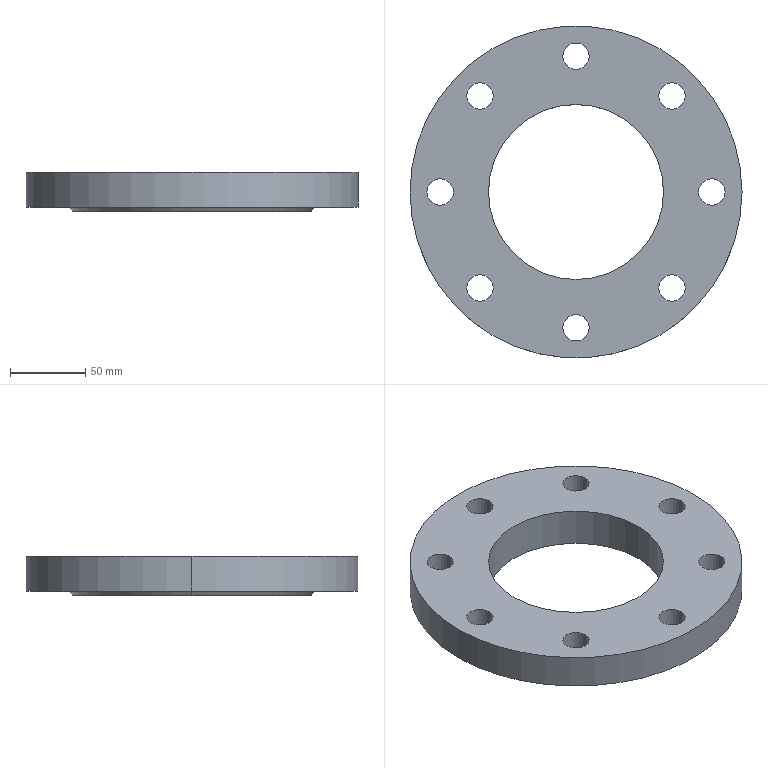Part | SolidWorks | features Extrusion 1, ICE 1, RefAxis 1, RevCut 1 | 1 solid | 25 faces | box 220 x 220 x 26 mm | volume 615594 mm3 | cylinder 20 | plane 3 | cone 2 | commonest cylinder face diameters 17.5 x16 116 x2 220 x2
STEP:
#1=CARTESIAN_POINT('',(-79.,0.,0.));
#2=VERTEX_POINT('',#1);
#3=CARTESIAN_POINT('',(79.,0.,0.));
#4=VERTEX_POINT('',#3);
#5=CARTESIAN_POINT('',(0.,0.,0.));
#6=DIRECTION('',(0.,0.,-1.));
#7=DIRECTION('',(-1.,0.,0.));
#8=AXIS2_PLACEMENT_3D('',#5,#6,#7);
#9=CIRCLE('',#8,79.);
#10=EDGE_CURVE('',#2,#4,#9,.T.);
#11=ORIENTED_EDGE('',*,*,#10,.F.);
#12=CARTESIAN_POINT('',(-81.,0.,3.));
#13=VERTEX_POINT('',#12);
#14=CARTESIAN_POINT('',(-79.,0.,0.));
#15=DIRECTION('',(-0.5547,0.,0.8321));
#16=VECTOR('',#15,1000.);
#17=LINE('',#14,#16);
#18=EDGE_CURVE('',#2,#13,#17,.T.);
#19=ORIENTED_EDGE('',*,*,#18,.T.);
#20=CARTESIAN_POINT('',(81.,0.,3.));
#21=VERTEX_POINT('',#20);
#22=CARTESIAN_POINT('',(0.,0.,3.));
#23=DIRECTION('',(0.,0.,-1.));
#24=DIRECTION('',(-1.,0.,0.));
#25=AXIS2_PLACEMENT_3D('',#22,#23,#24);
#26=CIRCLE('',#25,81.);
#27=EDGE_CURVE('',#13,#21,#26,.T.);
#28=ORIENTED_EDGE('',*,*,#27,.T.);
#29=CARTESIAN_POINT('',(79.,0.,0.));
#30=DIRECTION('',(0.5547,0.,0.8321));
#31=VECTOR('',#30,1000.);
#32=LINE('',#29,#31);
#33=EDGE_CURVE('',#4,#21,#32,.T.);
#34=ORIENTED_EDGE('',*,*,#33,.F.);
#35=EDGE_LOOP('',(#11,#19,#28,#34));
#36=FACE_OUTER_BOUND('',#35,.T.);
#37=CARTESIAN_POINT('',(0.,0.,0.));
#38=DIRECTION('',(0.,0.,1.));
#39=DIRECTION('',(1.,0.,0.));
#40=AXIS2_PLACEMENT_3D('',#37,#38,#39);
#41=CONICAL_SURFACE('',#40,79.,0.588);
#42=ADVANCED_FACE('',(#36),#41,.T.);
#43=CARTESIAN_POINT('',(-58.,0.,0.));
#44=VERTEX_POINT('',#43);
#45=CARTESIAN_POINT('',(58.,0.,0.));
#46=VERTEX_POINT('',#45);
#47=CARTESIAN_POINT('',(0.,0.,0.));
#48=DIRECTION('',(0.,0.,1.));
#49=DIRECTION('',(1.,0.,0.));
#50=AXIS2_PLACEMENT_3D('',#47,#48,#49);
#51=CIRCLE('',#50,58.);
#52=EDGE_CURVE('',#44,#46,#51,.T.);
#53=ORIENTED_EDGE('',*,*,#52,.F.);
#54=CARTESIAN_POINT('',(-58.,0.,26.));
#55=VERTEX_POINT('',#54);
#56=CARTESIAN_POINT('',(-58.,0.,0.));
#57=DIRECTION('',(0.,0.,1.));
#58=VECTOR('',#57,1000.);
#59=LINE('',#56,#58);
#60=EDGE_CURVE('',#44,#55,#59,.T.);
#61=ORIENTED_EDGE('',*,*,#60,.T.);
#62=CARTESIAN_POINT('',(58.,0.,26.));
#63=VERTEX_POINT('',#62);
#64=CARTESIAN_POINT('',(0.,0.,26.));
#65=DIRECTION('',(0.,0.,1.));
#66=DIRECTION('',(1.,0.,0.));
#67=AXIS2_PLACEMENT_3D('',#64,#65,#66);
#68=CIRCLE('',#67,58.);
#69=EDGE_CURVE('',#55,#63,#68,.T.);
#70=ORIENTED_EDGE('',*,*,#69,.T.);
#71=CARTESIAN_POINT('',(58.,0.,0.));
#72=DIRECTION('',(0.,0.,1.));
#73=VECTOR('',#72,1000.);
#74=LINE('',#71,#73);
#75=EDGE_CURVE('',#46,#63,#74,.T.);
#76=ORIENTED_EDGE('',*,*,#75,.F.);
#77=EDGE_LOOP('',(#53,#61,#70,#76));
#78=FACE_OUTER_BOUND('',#77,.T.);
#79=CARTESIAN_POINT('',(0.,0.,0.));
#80=DIRECTION('',(0.,0.,1.));
#81=DIRECTION('',(1.,0.,0.));
#82=AXIS2_PLACEMENT_3D('',#79,#80,#81);
#83=CYLINDRICAL_SURFACE('',#82,58.);
#84=ADVANCED_FACE('',(#78),#83,.F.);
#85=CARTESIAN_POINT('',(-72.39,63.64,26.));
#86=VERTEX_POINT('',#85);
#87=CARTESIAN_POINT('',(-54.89,63.64,26.));
#88=VERTEX_POINT('',#87);
#89=CARTESIAN_POINT('',(-63.64,63.64,26.));
#90=DIRECTION('',(0.,0.,1.));
#91=DIRECTION('',(1.,0.,0.));
#92=AXIS2_PLACEMENT_3D('',#89,#90,#91);
#93=CIRCLE('',#92,8.75);
#94=EDGE_CURVE('',#86,#88,#93,.T.);
#95=ORIENTED_EDGE('',*,*,#94,.T.);
#96=CARTESIAN_POINT('',(-54.89,63.64,3.));
#97=VERTEX_POINT('',#96);
#98=CARTESIAN_POINT('',(-54.89,63.64,26.));
#99=DIRECTION('',(0.,0.,-1.));
#100=VECTOR('',#99,1000.);
#101=LINE('',#98,#100);
#102=EDGE_CURVE('',#88,#97,#101,.T.);
#103=ORIENTED_EDGE('',*,*,#102,.T.);
#104=CARTESIAN_POINT('',(-72.39,63.64,3.));
#105=VERTEX_POINT('',#104);
#106=CARTESIAN_POINT('',(-63.64,63.64,3.));
#107=DIRECTION('',(0.,0.,-1.));
#108=DIRECTION('',(-1.,0.,0.));
#109=AXIS2_PLACEMENT_3D('',#106,#107,#108);
#110=CIRCLE('',#109,8.75);
#111=EDGE_CURVE('',#97,#105,#110,.T.);
#112=ORIENTED_EDGE('',*,*,#111,.T.);
#113=CARTESIAN_POINT('',(-72.39,63.64,26.));
#114=DIRECTION('',(0.,0.,-1.));
#115=VECTOR('',#114,1000.);
#116=LINE('',#113,#115);
#117=EDGE_CURVE('',#86,#105,#116,.T.);
#118=ORIENTED_EDGE('',*,*,#117,.F.);
#119=EDGE_LOOP('',(#95,#103,#112,#118));
#120=FACE_OUTER_BOUND('',#119,.T.);
#121=CARTESIAN_POINT('',(-63.64,63.64,26.));
#122=DIRECTION('',(0.,0.,-1.));
#123=DIRECTION('',(-1.,0.,0.));
#124=AXIS2_PLACEMENT_3D('',#121,#122,#123);
#125=CYLINDRICAL_SURFACE('',#124,8.75);
#126=ADVANCED_FACE('',(#120),#125,.F.);
#127=CARTESIAN_POINT('',(-98.75,0.,26.));
#128=VERTEX_POINT('',#127);
#129=CARTESIAN_POINT('',(-81.25,0.,26.));
#130=VERTEX_POINT('',#129);
#131=CARTESIAN_POINT('',(-90.,0.,26.));
#132=DIRECTION('',(0.,0.,1.));
#133=DIRECTION('',(1.,0.,0.));
#134=AXIS2_PLACEMENT_3D('',#131,#132,#133);
#135=CIRCLE('',#134,8.75);
#136=EDGE_CURVE('',#128,#130,#135,.T.);
#137=ORIENTED_EDGE('',*,*,#136,.T.);
#138=CARTESIAN_POINT('',(-81.25,0.,3.));
#139=VERTEX_POINT('',#138);
#140=CARTESIAN_POINT('',(-81.25,0.,26.));
#141=DIRECTION('',(0.,0.,-1.));
#142=VECTOR('',#141,1000.);
#143=LINE('',#140,#142);
#144=EDGE_CURVE('',#130,#139,#143,.T.);
#145=ORIENTED_EDGE('',*,*,#144,.T.);
#146=CARTESIAN_POINT('',(-98.75,0.,3.));
#147=VERTEX_POINT('',#146);
#148=CARTESIAN_POINT('',(-90.,0.,3.));
#149=DIRECTION('',(0.,0.,-1.));
#150=DIRECTION('',(-1.,0.,0.));
#151=AXIS2_PLACEMENT_3D('',#148,#149,#150);
#152=CIRCLE('',#151,8.75);
#153=EDGE_CURVE('',#139,#147,#152,.T.);
#154=ORIENTED_EDGE('',*,*,#153,.T.);
#155=CARTESIAN_POINT('',(-98.75,0.,26.));
#156=DIRECTION('',(0.,0.,-1.));
#157=VECTOR('',#156,1000.);
#158=LINE('',#155,#157);
#159=EDGE_CURVE('',#128,#147,#158,.T.);
#160=ORIENTED_EDGE('',*,*,#159,.F.);
#161=EDGE_LOOP('',(#137,#145,#154,#160));
#162=FACE_OUTER_BOUND('',#161,.T.);
#163=CARTESIAN_POINT('',(-90.,0.,26.));
#164=DIRECTION('',(0.,0.,-1.));
#165=DIRECTION('',(-1.,0.,0.));
#166=AXIS2_PLACEMENT_3D('',#163,#164,#165);
#167=CYLINDRICAL_SURFACE('',#166,8.75);
#168=ADVANCED_FACE('',(#162),#167,.F.);
#169=CARTESIAN_POINT('',(-72.39,-63.64,26.));
#170=VERTEX_POINT('',#169);
#171=CARTESIAN_POINT('',(-54.89,-63.64,26.));
#172=VERTEX_POINT('',#171);
#173=CARTESIAN_POINT('',(-63.64,-63.64,26.));
#174=DIRECTION('',(0.,0.,1.));
#175=DIRECTION('',(1.,0.,0.));
#176=AXIS2_PLACEMENT_3D('',#173,#174,#175);
#177=CIRCLE('',#176,8.75);
#178=EDGE_CURVE('',#170,#172,#177,.T.);
#179=ORIENTED_EDGE('',*,*,#178,.T.);
#180=CARTESIAN_POINT('',(-54.89,-63.64,3.));
#181=VERTEX_POINT('',#180);
#182=CARTESIAN_POINT('',(-54.89,-63.64,26.));
#183=DIRECTION('',(0.,0.,-1.));
#184=VECTOR('',#183,1000.);
#185=LINE('',#182,#184);
#186=EDGE_CURVE('',#172,#181,#185,.T.);
#187=ORIENTED_EDGE('',*,*,#186,.T.);
#188=CARTESIAN_POINT('',(-72.39,-63.64,3.));
#189=VERTEX_POINT('',#188);
#190=CARTESIAN_POINT('',(-63.64,-63.64,3.));
#191=DIRECTION('',(0.,0.,-1.));
#192=DIRECTION('',(-1.,0.,0.));
#193=AXIS2_PLACEMENT_3D('',#190,#191,#192);
#194=CIRCLE('',#193,8.75);
#195=EDGE_CURVE('',#181,#189,#194,.T.);
#196=ORIENTED_EDGE('',*,*,#195,.T.);
#197=CARTESIAN_POINT('',(-72.39,-63.64,26.));
#198=DIRECTION('',(0.,0.,-1.));
#199=VECTOR('',#198,1000.);
#200=LINE('',#197,#199);
#201=EDGE_CURVE('',#170,#189,#200,.T.);
#202=ORIENTED_EDGE('',*,*,#201,.F.);
#203=EDGE_LOOP('',(#179,#187,#196,#202));
#204=FACE_OUTER_BOUND('',#203,.T.);
#205=CARTESIAN_POINT('',(-63.64,-63.64,26.));
#206=DIRECTION('',(0.,0.,-1.));
#207=DIRECTION('',(-1.,0.,0.));
#208=AXIS2_PLACEMENT_3D('',#205,#206,#207);
#209=CYLINDRICAL_SURFACE('',#208,8.75);
#210=ADVANCED_FACE('',(#204),#209,.F.);
#211=CARTESIAN_POINT('',(-8.75,-90.,26.));
#212=VERTEX_POINT('',#211);
#213=CARTESIAN_POINT('',(8.75,-90.,26.));
#214=VERTEX_POINT('',#213);
#215=CARTESIAN_POINT('',(0.,-90.,26.));
#216=DIRECTION('',(0.,0.,1.));
#217=DIRECTION('',(1.,0.,0.));
#218=AXIS2_PLACEMENT_3D('',#215,#216,#217);
#219=CIRCLE('',#218,8.75);
#220=EDGE_CURVE('',#212,#214,#219,.T.);
#221=ORIENTED_EDGE('',*,*,#220,.T.);
#222=CARTESIAN_POINT('',(8.75,-90.,3.));
#223=VERTEX_POINT('',#222);
#224=CARTESIAN_POINT('',(8.75,-90.,26.));
#225=DIRECTION('',(0.,0.,-1.));
#226=VECTOR('',#225,1000.);
#227=LINE('',#224,#226);
#228=EDGE_CURVE('',#214,#223,#227,.T.);
#229=ORIENTED_EDGE('',*,*,#228,.T.);
#230=CARTESIAN_POINT('',(-8.75,-90.,3.));
#231=VERTEX_POINT('',#230);
#232=CARTESIAN_POINT('',(0.,-90.,3.));
#233=DIRECTION('',(0.,0.,-1.));
#234=DIRECTION('',(-1.,0.,0.));
#235=AXIS2_PLACEMENT_3D('',#232,#233,#234);
#236=CIRCLE('',#235,8.75);
#237=EDGE_CURVE('',#223,#231,#236,.T.);
#238=ORIENTED_EDGE('',*,*,#237,.T.);
#239=CARTESIAN_POINT('',(-8.75,-90.,26.));
#240=DIRECTION('',(0.,0.,-1.));
#241=VECTOR('',#240,1000.);
#242=LINE('',#239,#241);
#243=EDGE_CURVE('',#212,#231,#242,.T.);
#244=ORIENTED_EDGE('',*,*,#243,.F.);
#245=EDGE_LOOP('',(#221,#229,#238,#244));
#246=FACE_OUTER_BOUND('',#245,.T.);
#247=CARTESIAN_POINT('',(0.,-90.,26.));
#248=DIRECTION('',(0.,0.,-1.));
#249=DIRECTION('',(-1.,0.,0.));
#250=AXIS2_PLACEMENT_3D('',#247,#248,#249);
#251=CYLINDRICAL_SURFACE('',#250,8.75);
#252=ADVANCED_FACE('',(#246),#251,.F.);
#253=CARTESIAN_POINT('',(54.89,-63.64,26.));
#254=VERTEX_POINT('',#253);
#255=CARTESIAN_POINT('',(72.39,-63.64,26.));
#256=VERTEX_POINT('',#255);
#257=CARTESIAN_POINT('',(63.64,-63.64,26.));
#258=DIRECTION('',(0.,0.,1.));
#259=DIRECTION('',(1.,0.,0.));
#260=AXIS2_PLACEMENT_3D('',#257,#258,#259);
#261=CIRCLE('',#260,8.75);
#262=EDGE_CURVE('',#254,#256,#261,.T.);
#263=ORIENTED_EDGE('',*,*,#262,.T.);
#264=CARTESIAN_POINT('',(72.39,-63.64,3.));
#265=VERTEX_POINT('',#264);
#266=CARTESIAN_POINT('',(72.39,-63.64,26.));
#267=DIRECTION('',(0.,0.,-1.));
#268=VECTOR('',#267,1000.);
#269=LINE('',#266,#268);
#270=EDGE_CURVE('',#256,#265,#269,.T.);
#271=ORIENTED_EDGE('',*,*,#270,.T.);
#272=CARTESIAN_POINT('',(54.89,-63.64,3.));
#273=VERTEX_POINT('',#272);
#274=CARTESIAN_POINT('',(63.64,-63.64,3.));
#275=DIRECTION('',(0.,0.,-1.));
#276=DIRECTION('',(-1.,0.,0.));
#277=AXIS2_PLACEMENT_3D('',#274,#275,#276);
#278=CIRCLE('',#277,8.75);
#279=EDGE_CURVE('',#265,#273,#278,.T.);
#280=ORIENTED_EDGE('',*,*,#279,.T.);
#281=CARTESIAN_POINT('',(54.89,-63.64,26.));
#282=DIRECTION('',(0.,0.,-1.));
#283=VECTOR('',#282,1000.);
#284=LINE('',#281,#283);
#285=EDGE_CURVE('',#254,#273,#284,.T.);
#286=ORIENTED_EDGE('',*,*,#285,.F.);
#287=EDGE_LOOP('',(#263,#271,#280,#286));
#288=FACE_OUTER_BOUND('',#287,.T.);
#289=CARTESIAN_POINT('',(63.64,-63.64,26.));
#290=DIRECTION('',(0.,0.,-1.));
#291=DIRECTION('',(-1.,0.,0.));
#292=AXIS2_PLACEMENT_3D('',#289,#290,#291);
#293=CYLINDRICAL_SURFACE('',#292,8.75);
#294=ADVANCED_FACE('',(#288),#293,.F.);
#295=CARTESIAN_POINT('',(81.25,0.,26.));
#296=VERTEX_POINT('',#295);
#297=CARTESIAN_POINT('',(98.75,0.,26.));
#298=VERTEX_POINT('',#297);
#299=CARTESIAN_POINT('',(90.,0.,26.));
#300=DIRECTION('',(0.,0.,1.));
#301=DIRECTION('',(1.,0.,0.));
#302=AXIS2_PLACEMENT_3D('',#299,#300,#301);
#303=CIRCLE('',#302,8.75);
#304=EDGE_CURVE('',#296,#298,#303,.T.);
#305=ORIENTED_EDGE('',*,*,#304,.T.);
#306=CARTESIAN_POINT('',(98.75,0.,3.));
#307=VERTEX_POINT('',#306);
#308=CARTESIAN_POINT('',(98.75,0.,26.));
#309=DIRECTION('',(0.,0.,-1.));
#310=VECTOR('',#309,1000.);
#311=LINE('',#308,#310);
#312=EDGE_CURVE('',#298,#307,#311,.T.);
#313=ORIENTED_EDGE('',*,*,#312,.T.);
#314=CARTESIAN_POINT('',(81.25,0.,3.));
#315=VERTEX_POINT('',#314);
#316=CARTESIAN_POINT('',(90.,0.,3.));
#317=DIRECTION('',(0.,0.,-1.));
#318=DIRECTION('',(-1.,0.,0.));
#319=AXIS2_PLACEMENT_3D('',#316,#317,#318);
#320=CIRCLE('',#319,8.75);
#321=EDGE_CURVE('',#307,#315,#320,.T.);
#322=ORIENTED_EDGE('',*,*,#321,.T.);
#323=CARTESIAN_POINT('',(81.25,0.,26.));
#324=DIRECTION('',(0.,0.,-1.));
#325=VECTOR('',#324,1000.);
#326=LINE('',#323,#325);
#327=EDGE_CURVE('',#296,#315,#326,.T.);
#328=ORIENTED_EDGE('',*,*,#327,.F.);
#329=EDGE_LOOP('',(#305,#313,#322,#328));
#330=FACE_OUTER_BOUND('',#329,.T.);
#331=CARTESIAN_POINT('',(90.,0.,26.));
#332=DIRECTION('',(0.,0.,-1.));
#333=DIRECTION('',(-1.,0.,0.));
#334=AXIS2_PLACEMENT_3D('',#331,#332,#333);
#335=CYLINDRICAL_SURFACE('',#334,8.75);
#336=ADVANCED_FACE('',(#330),#335,.F.);
#337=CARTESIAN_POINT('',(54.89,63.64,26.));
#338=VERTEX_POINT('',#337);
#339=CARTESIAN_POINT('',(72.39,63.64,26.));
#340=VERTEX_POINT('',#339);
#341=CARTESIAN_POINT('',(63.64,63.64,26.));
#342=DIRECTION('',(0.,0.,1.));
#343=DIRECTION('',(1.,0.,0.));
#344=AXIS2_PLACEMENT_3D('',#341,#342,#343);
#345=CIRCLE('',#344,8.75);
#346=EDGE_CURVE('',#338,#340,#345,.T.);
#347=ORIENTED_EDGE('',*,*,#346,.T.);
#348=CARTESIAN_POINT('',(72.39,63.64,3.));
#349=VERTEX_POINT('',#348);
#350=CARTESIAN_POINT('',(72.39,63.64,26.));
#351=DIRECTION('',(0.,0.,-1.));
#352=VECTOR('',#351,1000.);
#353=LINE('',#350,#352);
#354=EDGE_CURVE('',#340,#349,#353,.T.);
#355=ORIENTED_EDGE('',*,*,#354,.T.);
#356=CARTESIAN_POINT('',(54.89,63.64,3.));
#357=VERTEX_POINT('',#356);
#358=CARTESIAN_POINT('',(63.64,63.64,3.));
#359=DIRECTION('',(0.,0.,-1.));
#360=DIRECTION('',(-1.,0.,0.));
#361=AXIS2_PLACEMENT_3D('',#358,#359,#360);
#362=CIRCLE('',#361,8.75);
#363=EDGE_CURVE('',#349,#357,#362,.T.);
#364=ORIENTED_EDGE('',*,*,#363,.T.);
#365=CARTESIAN_POINT('',(54.89,63.64,26.));
#366=DIRECTION('',(0.,0.,-1.));
#367=VECTOR('',#366,1000.);
#368=LINE('',#365,#367);
#369=EDGE_CURVE('',#338,#357,#368,.T.);
#370=ORIENTED_EDGE('',*,*,#369,.F.);
#371=EDGE_LOOP('',(#347,#355,#364,#370));
#372=FACE_OUTER_BOUND('',#371,.T.);
#373=CARTESIAN_POINT('',(63.64,63.64,26.));
#374=DIRECTION('',(0.,0.,-1.));
#375=DIRECTION('',(-1.,0.,0.));
#376=AXIS2_PLACEMENT_3D('',#373,#374,#375);
#377=CYLINDRICAL_SURFACE('',#376,8.75);
#378=ADVANCED_FACE('',(#372),#377,.F.);
#379=CARTESIAN_POINT('',(-8.75,90.,26.));
#380=VERTEX_POINT('',#379);
#381=CARTESIAN_POINT('',(8.75,90.,26.));
#382=VERTEX_POINT('',#381);
#383=CARTESIAN_POINT('',(0.,90.,26.));
#384=DIRECTION('',(0.,0.,1.));
#385=DIRECTION('',(1.,0.,0.));
#386=AXIS2_PLACEMENT_3D('',#383,#384,#385);
#387=CIRCLE('',#386,8.75);
#388=EDGE_CURVE('',#380,#382,#387,.T.);
#389=ORIENTED_EDGE('',*,*,#388,.T.);
#390=CARTESIAN_POINT('',(8.75,90.,3.));
#391=VERTEX_POINT('',#390);
#392=CARTESIAN_POINT('',(8.75,90.,26.));
#393=DIRECTION('',(0.,0.,-1.));
#394=VECTOR('',#393,1000.);
#395=LINE('',#392,#394);
#396=EDGE_CURVE('',#382,#391,#395,.T.);
#397=ORIENTED_EDGE('',*,*,#396,.T.);
#398=CARTESIAN_POINT('',(-8.75,90.,3.));
#399=VERTEX_POINT('',#398);
#400=CARTESIAN_POINT('',(0.,90.,3.));
#401=DIRECTION('',(0.,0.,-1.));
#402=DIRECTION('',(-1.,0.,0.));
#403=AXIS2_PLACEMENT_3D('',#400,#401,#402);
#404=CIRCLE('',#403,8.75);
#405=EDGE_CURVE('',#391,#399,#404,.T.);
#406=ORIENTED_EDGE('',*,*,#405,.T.);
#407=CARTESIAN_POINT('',(-8.75,90.,26.));
#408=DIRECTION('',(0.,0.,-1.));
#409=VECTOR('',#408,1000.);
#410=LINE('',#407,#409);
#411=EDGE_CURVE('',#380,#399,#410,.T.);
#412=ORIENTED_EDGE('',*,*,#411,.F.);
#413=EDGE_LOOP('',(#389,#397,#406,#412));
#414=FACE_OUTER_BOUND('',#413,.T.);
#415=CARTESIAN_POINT('',(0.,90.,26.));
#416=DIRECTION('',(0.,0.,-1.));
#417=DIRECTION('',(-1.,0.,0.));
#418=AXIS2_PLACEMENT_3D('',#415,#416,#417);
#419=CYLINDRICAL_SURFACE('',#418,8.75);
#420=ADVANCED_FACE('',(#414),#419,.F.);
#421=CARTESIAN_POINT('',(110.,0.,26.));
#422=VERTEX_POINT('',#421);
#423=CARTESIAN_POINT('',(-110.,0.,26.));
#424=VERTEX_POINT('',#423);
#425=CARTESIAN_POINT('',(0.,0.,26.));
#426=DIRECTION('',(0.,0.,1.));
#427=DIRECTION('',(1.,0.,0.));
#428=AXIS2_PLACEMENT_3D('',#425,#426,#427);
#429=CIRCLE('',#428,110.);
#430=EDGE_CURVE('',#422,#424,#429,.T.);
#431=ORIENTED_EDGE('',*,*,#430,.F.);
#432=CARTESIAN_POINT('',(110.,0.,3.));
#433=VERTEX_POINT('',#432);
#434=CARTESIAN_POINT('',(110.,0.,26.));
#435=DIRECTION('',(0.,0.,-1.));
#436=VECTOR('',#435,1000.);
#437=LINE('',#434,#436);
#438=EDGE_CURVE('',#422,#433,#437,.T.);
#439=ORIENTED_EDGE('',*,*,#438,.T.);
#440=CARTESIAN_POINT('',(-110.,0.,3.));
#441=VERTEX_POINT('',#440);
#442=CARTESIAN_POINT('',(0.,0.,3.));
#443=DIRECTION('',(0.,0.,-1.));
#444=DIRECTION('',(-1.,0.,0.));
#445=AXIS2_PLACEMENT_3D('',#442,#443,#444);
#446=CIRCLE('',#445,110.);
#447=EDGE_CURVE('',#441,#433,#446,.T.);
#448=ORIENTED_EDGE('',*,*,#447,.F.);
#449=CARTESIAN_POINT('',(-110.,0.,26.));
#450=DIRECTION('',(0.,0.,-1.));
#451=VECTOR('',#450,1000.);
#452=LINE('',#449,#451);
#453=EDGE_CURVE('',#424,#441,#452,.T.);
#454=ORIENTED_EDGE('',*,*,#453,.F.);
#455=EDGE_LOOP('',(#431,#439,#448,#454));
#456=FACE_OUTER_BOUND('',#455,.T.);
#457=CARTESIAN_POINT('',(0.,0.,26.));
#458=DIRECTION('',(0.,0.,-1.));
#459=DIRECTION('',(-1.,0.,0.));
#460=AXIS2_PLACEMENT_3D('',#457,#458,#459);
#461=CYLINDRICAL_SURFACE('',#460,110.);
#462=ADVANCED_FACE('',(#456),#461,.T.);
#463=CARTESIAN_POINT('',(0.,0.,0.));
#464=DIRECTION('',(0.,0.,1.));
#465=DIRECTION('',(1.,0.,0.));
#466=AXIS2_PLACEMENT_3D('',#463,#464,#465);
#467=CIRCLE('',#466,58.);
#468=EDGE_CURVE('',#46,#44,#467,.T.);
#469=ORIENTED_EDGE('',*,*,#468,.T.);
#470=ORIENTED_EDGE('',*,*,#52,.T.);
#471=EDGE_LOOP('',(#469,#470));
#472=FACE_BOUND('',#471,.T.);
#473=CARTESIAN_POINT('',(0.,0.,0.));
#474=DIRECTION('',(0.,0.,-1.));
#475=DIRECTION('',(-1.,0.,0.));
#476=AXIS2_PLACEMENT_3D('',#473,#474,#475);
#477=CIRCLE('',#476,79.);
#478=EDGE_CURVE('',#4,#2,#477,.T.);
#479=ORIENTED_EDGE('',*,*,#478,.T.);
#480=ORIENTED_EDGE('',*,*,#10,.T.);
#481=EDGE_LOOP('',(#479,#480));
#482=FACE_OUTER_BOUND('',#481,.T.);
#483=CARTESIAN_POINT('',(0.,0.,0.));
#484=DIRECTION('',(0.,0.,1.));
#485=DIRECTION('',(1.,0.,0.));
#486=AXIS2_PLACEMENT_3D('',#483,#484,#485);
#487=PLANE('',#486);
#488=ADVANCED_FACE('',(#472,#482),#487,.F.);
#489=ORIENTED_EDGE('',*,*,#438,.F.);
#490=CARTESIAN_POINT('',(0.,0.,26.));
#491=DIRECTION('',(0.,0.,1.));
#492=DIRECTION('',(1.,0.,0.));
#493=AXIS2_PLACEMENT_3D('',#490,#491,#492);
#494=CIRCLE('',#493,110.);
#495=EDGE_CURVE('',#424,#422,#494,.T.);
#496=ORIENTED_EDGE('',*,*,#495,.F.);
#497=ORIENTED_EDGE('',*,*,#453,.T.);
#498=CARTESIAN_POINT('',(0.,0.,3.));
#499=DIRECTION('',(0.,0.,-1.));
#500=DIRECTION('',(-1.,0.,0.));
#501=AXIS2_PLACEMENT_3D('',#498,#499,#500);
#502=CIRCLE('',#501,110.);
#503=EDGE_CURVE('',#433,#441,#502,.T.);
#504=ORIENTED_EDGE('',*,*,#503,.F.);
#505=EDGE_LOOP('',(#489,#496,#497,#504));
#506=FACE_OUTER_BOUND('',#505,.T.);
#507=CARTESIAN_POINT('',(0.,0.,26.));
#508=DIRECTION('',(0.,0.,-1.));
#509=DIRECTION('',(-1.,0.,0.));
#510=AXIS2_PLACEMENT_3D('',#507,#508,#509);
#511=CYLINDRICAL_SURFACE('',#510,110.);
#512=ADVANCED_FACE('',(#506),#511,.T.);
#513=ORIENTED_EDGE('',*,*,#396,.F.);
#514=CARTESIAN_POINT('',(0.,90.,26.));
#515=DIRECTION('',(0.,0.,1.));
#516=DIRECTION('',(1.,0.,0.));
#517=AXIS2_PLACEMENT_3D('',#514,#515,#516);
#518=CIRCLE('',#517,8.75);
#519=EDGE_CURVE('',#382,#380,#518,.T.);
#520=ORIENTED_EDGE('',*,*,#519,.T.);
#521=ORIENTED_EDGE('',*,*,#411,.T.);
#522=CARTESIAN_POINT('',(0.,90.,3.));
#523=DIRECTION('',(0.,0.,-1.));
#524=DIRECTION('',(-1.,0.,0.));
#525=AXIS2_PLACEMENT_3D('',#522,#523,#524);
#526=CIRCLE('',#525,8.75);
#527=EDGE_CURVE('',#399,#391,#526,.T.);
#528=ORIENTED_EDGE('',*,*,#527,.T.);
#529=EDGE_LOOP('',(#513,#520,#521,#528));
#530=FACE_OUTER_BOUND('',#529,.T.);
#531=CARTESIAN_POINT('',(0.,90.,26.));
#532=DIRECTION('',(0.,0.,-1.));
#533=DIRECTION('',(-1.,0.,0.));
#534=AXIS2_PLACEMENT_3D('',#531,#532,#533);
#535=CYLINDRICAL_SURFACE('',#534,8.75);
#536=ADVANCED_FACE('',(#530),#535,.F.);
#537=ORIENTED_EDGE('',*,*,#354,.F.);
#538=CARTESIAN_POINT('',(63.64,63.64,26.));
#539=DIRECTION('',(0.,0.,1.));
#540=DIRECTION('',(1.,0.,0.));
#541=AXIS2_PLACEMENT_3D('',#538,#539,#540);
#542=CIRCLE('',#541,8.75);
#543=EDGE_CURVE('',#340,#338,#542,.T.);
#544=ORIENTED_EDGE('',*,*,#543,.T.);
#545=ORIENTED_EDGE('',*,*,#369,.T.);
#546=CARTESIAN_POINT('',(63.64,63.64,3.));
#547=DIRECTION('',(0.,0.,-1.));
#548=DIRECTION('',(-1.,0.,0.));
#549=AXIS2_PLACEMENT_3D('',#546,#547,#548);
#550=CIRCLE('',#549,8.75);
#551=EDGE_CURVE('',#357,#349,#550,.T.);
#552=ORIENTED_EDGE('',*,*,#551,.T.);
#553=EDGE_LOOP('',(#537,#544,#545,#552));
#554=FACE_OUTER_BOUND('',#553,.T.);
#555=CARTESIAN_POINT('',(63.64,63.64,26.));
#556=DIRECTION('',(0.,0.,-1.));
#557=DIRECTION('',(-1.,0.,0.));
#558=AXIS2_PLACEMENT_3D('',#555,#556,#557);
#559=CYLINDRICAL_SURFACE('',#558,8.75);
#560=ADVANCED_FACE('',(#554),#559,.F.);
#561=ORIENTED_EDGE('',*,*,#312,.F.);
#562=CARTESIAN_POINT('',(90.,0.,26.));
#563=DIRECTION('',(0.,0.,1.));
#564=DIRECTION('',(1.,0.,0.));
#565=AXIS2_PLACEMENT_3D('',#562,#563,#564);
#566=CIRCLE('',#565,8.75);
#567=EDGE_CURVE('',#298,#296,#566,.T.);
#568=ORIENTED_EDGE('',*,*,#567,.T.);
#569=ORIENTED_EDGE('',*,*,#327,.T.);
#570=CARTESIAN_POINT('',(90.,0.,3.));
#571=DIRECTION('',(0.,0.,-1.));
#572=DIRECTION('',(-1.,0.,0.));
#573=AXIS2_PLACEMENT_3D('',#570,#571,#572);
#574=CIRCLE('',#573,8.75);
#575=EDGE_CURVE('',#315,#307,#574,.T.);
#576=ORIENTED_EDGE('',*,*,#575,.T.);
#577=EDGE_LOOP('',(#561,#568,#569,#576));
#578=FACE_OUTER_BOUND('',#577,.T.);
#579=CARTESIAN_POINT('',(90.,0.,26.));
#580=DIRECTION('',(0.,0.,-1.));
#581=DIRECTION('',(-1.,0.,0.));
#582=AXIS2_PLACEMENT_3D('',#579,#580,#581);
#583=CYLINDRICAL_SURFACE('',#582,8.75);
#584=ADVANCED_FACE('',(#578),#583,.F.);
#585=ORIENTED_EDGE('',*,*,#270,.F.);
#586=CARTESIAN_POINT('',(63.64,-63.64,26.));
#587=DIRECTION('',(0.,0.,1.));
#588=DIRECTION('',(1.,0.,0.));
#589=AXIS2_PLACEMENT_3D('',#586,#587,#588);
#590=CIRCLE('',#589,8.75);
#591=EDGE_CURVE('',#256,#254,#590,.T.);
#592=ORIENTED_EDGE('',*,*,#591,.T.);
#593=ORIENTED_EDGE('',*,*,#285,.T.);
#594=CARTESIAN_POINT('',(63.64,-63.64,3.));
#595=DIRECTION('',(0.,0.,-1.));
#596=DIRECTION('',(-1.,0.,0.));
#597=AXIS2_PLACEMENT_3D('',#594,#595,#596);
#598=CIRCLE('',#597,8.75);
#599=EDGE_CURVE('',#273,#265,#598,.T.);
#600=ORIENTED_EDGE('',*,*,#599,.T.);
#601=EDGE_LOOP('',(#585,#592,#593,#600));
#602=FACE_OUTER_BOUND('',#601,.T.);
#603=CARTESIAN_POINT('',(63.64,-63.64,26.));
#604=DIRECTION('',(0.,0.,-1.));
#605=DIRECTION('',(-1.,0.,0.));
#606=AXIS2_PLACEMENT_3D('',#603,#604,#605);
#607=CYLINDRICAL_SURFACE('',#606,8.75);
#608=ADVANCED_FACE('',(#602),#607,.F.);
#609=ORIENTED_EDGE('',*,*,#228,.F.);
#610=CARTESIAN_POINT('',(0.,-90.,26.));
#611=DIRECTION('',(0.,0.,1.));
#612=DIRECTION('',(1.,0.,0.));
#613=AXIS2_PLACEMENT_3D('',#610,#611,#612);
#614=CIRCLE('',#613,8.75);
#615=EDGE_CURVE('',#214,#212,#614,.T.);
#616=ORIENTED_EDGE('',*,*,#615,.T.);
#617=ORIENTED_EDGE('',*,*,#243,.T.);
#618=CARTESIAN_POINT('',(0.,-90.,3.));
#619=DIRECTION('',(0.,0.,-1.));
#620=DIRECTION('',(-1.,0.,0.));
#621=AXIS2_PLACEMENT_3D('',#618,#619,#620);
#622=CIRCLE('',#621,8.75);
#623=EDGE_CURVE('',#231,#223,#622,.T.);
#624=ORIENTED_EDGE('',*,*,#623,.T.);
#625=EDGE_LOOP('',(#609,#616,#617,#624));
#626=FACE_OUTER_BOUND('',#625,.T.);
#627=CARTESIAN_POINT('',(0.,-90.,26.));
#628=DIRECTION('',(0.,0.,-1.));
#629=DIRECTION('',(-1.,0.,0.));
#630=AXIS2_PLACEMENT_3D('',#627,#628,#629);
#631=CYLINDRICAL_SURFACE('',#630,8.75);
#632=ADVANCED_FACE('',(#626),#631,.F.);
#633=ORIENTED_EDGE('',*,*,#186,.F.);
#634=CARTESIAN_POINT('',(-63.64,-63.64,26.));
#635=DIRECTION('',(0.,0.,1.));
#636=DIRECTION('',(1.,0.,0.));
#637=AXIS2_PLACEMENT_3D('',#634,#635,#636);
#638=CIRCLE('',#637,8.75);
#639=EDGE_CURVE('',#172,#170,#638,.T.);
#640=ORIENTED_EDGE('',*,*,#639,.T.);
#641=ORIENTED_EDGE('',*,*,#201,.T.);
#642=CARTESIAN_POINT('',(-63.64,-63.64,3.));
#643=DIRECTION('',(0.,0.,-1.));
#644=DIRECTION('',(-1.,0.,0.));
#645=AXIS2_PLACEMENT_3D('',#642,#643,#644);
#646=CIRCLE('',#645,8.75);
#647=EDGE_CURVE('',#189,#181,#646,.T.);
#648=ORIENTED_EDGE('',*,*,#647,.T.);
#649=EDGE_LOOP('',(#633,#640,#641,#648));
#650=FACE_OUTER_BOUND('',#649,.T.);
#651=CARTESIAN_POINT('',(-63.64,-63.64,26.));
#652=DIRECTION('',(0.,0.,-1.));
#653=DIRECTION('',(-1.,0.,0.));
#654=AXIS2_PLACEMENT_3D('',#651,#652,#653);
#655=CYLINDRICAL_SURFACE('',#654,8.75);
#656=ADVANCED_FACE('',(#650),#655,.F.);
#657=ORIENTED_EDGE('',*,*,#144,.F.);
#658=CARTESIAN_POINT('',(-90.,0.,26.));
#659=DIRECTION('',(0.,0.,1.));
#660=DIRECTION('',(1.,0.,0.));
#661=AXIS2_PLACEMENT_3D('',#658,#659,#660);
#662=CIRCLE('',#661,8.75);
#663=EDGE_CURVE('',#130,#128,#662,.T.);
#664=ORIENTED_EDGE('',*,*,#663,.T.);
#665=ORIENTED_EDGE('',*,*,#159,.T.);
#666=CARTESIAN_POINT('',(-90.,0.,3.));
#667=DIRECTION('',(0.,0.,-1.));
#668=DIRECTION('',(-1.,0.,0.));
#669=AXIS2_PLACEMENT_3D('',#666,#667,#668);
#670=CIRCLE('',#669,8.75);
#671=EDGE_CURVE('',#147,#139,#670,.T.);
#672=ORIENTED_EDGE('',*,*,#671,.T.);
#673=EDGE_LOOP('',(#657,#664,#665,#672));
#674=FACE_OUTER_BOUND('',#673,.T.);
#675=CARTESIAN_POINT('',(-90.,0.,26.));
#676=DIRECTION('',(0.,0.,-1.));
#677=DIRECTION('',(-1.,0.,0.));
#678=AXIS2_PLACEMENT_3D('',#675,#676,#677);
#679=CYLINDRICAL_SURFACE('',#678,8.75);
#680=ADVANCED_FACE('',(#674),#679,.F.);
#681=ORIENTED_EDGE('',*,*,#102,.F.);
#682=CARTESIAN_POINT('',(-63.64,63.64,26.));
#683=DIRECTION('',(0.,0.,1.));
#684=DIRECTION('',(1.,0.,0.));
#685=AXIS2_PLACEMENT_3D('',#682,#683,#684);
#686=CIRCLE('',#685,8.75);
#687=EDGE_CURVE('',#88,#86,#686,.T.);
#688=ORIENTED_EDGE('',*,*,#687,.T.);
#689=ORIENTED_EDGE('',*,*,#117,.T.);
#690=CARTESIAN_POINT('',(-63.64,63.64,3.));
#691=DIRECTION('',(0.,0.,-1.));
#692=DIRECTION('',(-1.,0.,0.));
#693=AXIS2_PLACEMENT_3D('',#690,#691,#692);
#694=CIRCLE('',#693,8.75);
#695=EDGE_CURVE('',#105,#97,#694,.T.);
#696=ORIENTED_EDGE('',*,*,#695,.T.);
#697=EDGE_LOOP('',(#681,#688,#689,#696));
#698=FACE_OUTER_BOUND('',#697,.T.);
#699=CARTESIAN_POINT('',(-63.64,63.64,26.));
#700=DIRECTION('',(0.,0.,-1.));
#701=DIRECTION('',(-1.,0.,0.));
#702=AXIS2_PLACEMENT_3D('',#699,#700,#701);
#703=CYLINDRICAL_SURFACE('',#702,8.75);
#704=ADVANCED_FACE('',(#698),#703,.F.);
#705=CARTESIAN_POINT('',(0.,0.,26.));
#706=DIRECTION('',(0.,0.,1.));
#707=DIRECTION('',(1.,0.,0.));
#708=AXIS2_PLACEMENT_3D('',#705,#706,#707);
#709=CIRCLE('',#708,58.);
#710=EDGE_CURVE('',#63,#55,#709,.T.);
#711=ORIENTED_EDGE('',*,*,#710,.F.);
#712=ORIENTED_EDGE('',*,*,#69,.F.);
#713=EDGE_LOOP('',(#711,#712));
#714=FACE_BOUND('',#713,.T.);
#715=ORIENTED_EDGE('',*,*,#136,.F.);
#716=ORIENTED_EDGE('',*,*,#663,.F.);
#717=EDGE_LOOP('',(#715,#716));
#718=FACE_BOUND('',#717,.T.);
#719=ORIENTED_EDGE('',*,*,#220,.F.);
#720=ORIENTED_EDGE('',*,*,#615,.F.);
#721=EDGE_LOOP('',(#719,#720));
#722=FACE_BOUND('',#721,.T.);
#723=ORIENTED_EDGE('',*,*,#304,.F.);
#724=ORIENTED_EDGE('',*,*,#567,.F.);
#725=EDGE_LOOP('',(#723,#724));
#726=FACE_BOUND('',#725,.T.);
#727=ORIENTED_EDGE('',*,*,#388,.F.);
#728=ORIENTED_EDGE('',*,*,#519,.F.);
#729=EDGE_LOOP('',(#727,#728));
#730=FACE_BOUND('',#729,.T.);
#731=ORIENTED_EDGE('',*,*,#495,.T.);
#732=ORIENTED_EDGE('',*,*,#430,.T.);
#733=EDGE_LOOP('',(#731,#732));
#734=FACE_OUTER_BOUND('',#733,.T.);
#735=ORIENTED_EDGE('',*,*,#346,.F.);
#736=ORIENTED_EDGE('',*,*,#543,.F.);
#737=EDGE_LOOP('',(#735,#736));
#738=FACE_BOUND('',#737,.T.);
#739=ORIENTED_EDGE('',*,*,#262,.F.);
#740=ORIENTED_EDGE('',*,*,#591,.F.);
#741=EDGE_LOOP('',(#739,#740));
#742=FACE_BOUND('',#741,.T.);
#743=ORIENTED_EDGE('',*,*,#178,.F.);
#744=ORIENTED_EDGE('',*,*,#639,.F.);
#745=EDGE_LOOP('',(#743,#744));
#746=FACE_BOUND('',#745,.T.);
#747=ORIENTED_EDGE('',*,*,#94,.F.);
#748=ORIENTED_EDGE('',*,*,#687,.F.);
#749=EDGE_LOOP('',(#747,#748));
#750=FACE_BOUND('',#749,.T.);
#751=CARTESIAN_POINT('',(0.,0.,26.));
#752=DIRECTION('',(0.,0.,1.));
#753=DIRECTION('',(1.,0.,0.));
#754=AXIS2_PLACEMENT_3D('',#751,#752,#753);
#755=PLANE('',#754);
#756=ADVANCED_FACE('',(#714,#718,#722,#726,#730,#734,#738,#742,#746,#750),#755,.T.);
#757=ORIENTED_EDGE('',*,*,#60,.F.);
#758=ORIENTED_EDGE('',*,*,#468,.F.);
#759=ORIENTED_EDGE('',*,*,#75,.T.);
#760=ORIENTED_EDGE('',*,*,#710,.T.);
#761=EDGE_LOOP('',(#757,#758,#759,#760));
#762=FACE_OUTER_BOUND('',#761,.T.);
#763=CARTESIAN_POINT('',(0.,0.,0.));
#764=DIRECTION('',(0.,0.,1.));
#765=DIRECTION('',(1.,0.,0.));
#766=AXIS2_PLACEMENT_3D('',#763,#764,#765);
#767=CYLINDRICAL_SURFACE('',#766,58.);
#768=ADVANCED_FACE('',(#762),#767,.F.);
#769=ORIENTED_EDGE('',*,*,#527,.F.);
#770=ORIENTED_EDGE('',*,*,#405,.F.);
#771=EDGE_LOOP('',(#769,#770));
#772=FACE_BOUND('',#771,.T.);
#773=ORIENTED_EDGE('',*,*,#551,.F.);
#774=ORIENTED_EDGE('',*,*,#363,.F.);
#775=EDGE_LOOP('',(#773,#774));
#776=FACE_BOUND('',#775,.T.);
#777=ORIENTED_EDGE('',*,*,#575,.F.);
#778=ORIENTED_EDGE('',*,*,#321,.F.);
#779=EDGE_LOOP('',(#777,#778));
#780=FACE_BOUND('',#779,.T.);
#781=ORIENTED_EDGE('',*,*,#599,.F.);
#782=ORIENTED_EDGE('',*,*,#279,.F.);
#783=EDGE_LOOP('',(#781,#782));
#784=FACE_BOUND('',#783,.T.);
#785=ORIENTED_EDGE('',*,*,#623,.F.);
#786=ORIENTED_EDGE('',*,*,#237,.F.);
#787=EDGE_LOOP('',(#785,#786));
#788=FACE_BOUND('',#787,.T.);
#789=ORIENTED_EDGE('',*,*,#647,.F.);
#790=ORIENTED_EDGE('',*,*,#195,.F.);
#791=EDGE_LOOP('',(#789,#790));
#792=FACE_BOUND('',#791,.T.);
#793=ORIENTED_EDGE('',*,*,#671,.F.);
#794=ORIENTED_EDGE('',*,*,#153,.F.);
#795=EDGE_LOOP('',(#793,#794));
#796=FACE_BOUND('',#795,.T.);
#797=ORIENTED_EDGE('',*,*,#695,.F.);
#798=ORIENTED_EDGE('',*,*,#111,.F.);
#799=EDGE_LOOP('',(#797,#798));
#800=FACE_BOUND('',#799,.T.);
#801=ORIENTED_EDGE('',*,*,#447,.T.);
#802=ORIENTED_EDGE('',*,*,#503,.T.);
#803=EDGE_LOOP('',(#801,#802));
#804=FACE_OUTER_BOUND('',#803,.T.);
#805=CARTESIAN_POINT('',(0.,0.,3.));
#806=DIRECTION('',(0.,0.,-1.));
#807=DIRECTION('',(-1.,0.,0.));
#808=AXIS2_PLACEMENT_3D('',#805,#806,#807);
#809=CIRCLE('',#808,81.);
#810=EDGE_CURVE('',#21,#13,#809,.T.);
#811=ORIENTED_EDGE('',*,*,#810,.F.);
#812=ORIENTED_EDGE('',*,*,#27,.F.);
#813=EDGE_LOOP('',(#811,#812));
#814=FACE_BOUND('',#813,.T.);
#815=CARTESIAN_POINT('',(81.,0.,3.));
#816=DIRECTION('',(0.,0.,-1.));
#817=DIRECTION('',(-1.,0.,0.));
#818=AXIS2_PLACEMENT_3D('',#815,#816,#817);
#819=PLANE('',#818);
#820=ADVANCED_FACE('',(#772,#776,#780,#784,#788,#792,#796,#800,#804,#814),#819,.T.);
#821=ORIENTED_EDGE('',*,*,#18,.F.);
#822=ORIENTED_EDGE('',*,*,#478,.F.);
#823=ORIENTED_EDGE('',*,*,#33,.T.);
#824=ORIENTED_EDGE('',*,*,#810,.T.);
#825=EDGE_LOOP('',(#821,#822,#823,#824));
#826=FACE_OUTER_BOUND('',#825,.T.);
#827=CARTESIAN_POINT('',(0.,0.,0.));
#828=DIRECTION('',(0.,0.,1.));
#829=DIRECTION('',(1.,0.,0.));
#830=AXIS2_PLACEMENT_3D('',#827,#828,#829);
#831=CONICAL_SURFACE('',#830,79.,0.588);
#832=ADVANCED_FACE('',(#826),#831,.T.);
#833=CLOSED_SHELL('',(#42,#84,#126,#168,#210,#252,#294,#336,#378,#420,#462,#488,#512,#536,#560,#584,#608,#632,#656,#680,#704,#756,#768,#820,#832));
#834=MANIFOLD_SOLID_BREP('',#833);
#835=CARTESIAN_POINT('',(0.,0.,0.));
#836=DIRECTION('',(0.,0.,1.));
#837=DIRECTION('',(1.,0.,0.));
#838=AXIS2_PLACEMENT_3D('',#835,#836,#837);
#839=(LENGTH_UNIT()NAMED_UNIT(*)SI_UNIT(.MILLI.,.METRE.));
#840=UNCERTAINTY_MEASURE_WITH_UNIT(LENGTH_MEASURE(0.00001),#839,'','');
#841=(NAMED_UNIT(*)PLANE_ANGLE_UNIT()SI_UNIT($,.RADIAN.));
#842=(NAMED_UNIT(*)SI_UNIT($,.STERADIAN.)SOLID_ANGLE_UNIT());
#843=(GEOMETRIC_REPRESENTATION_CONTEXT(3)GLOBAL_UNCERTAINTY_ASSIGNED_CONTEXT((#840))GLOBAL_UNIT_ASSIGNED_CONTEXT((#839,#841,#842))REPRESENTATION_CONTEXT('',''));
#844=ADVANCED_BREP_SHAPE_REPRESENTATION('',(#834,#838),#843);